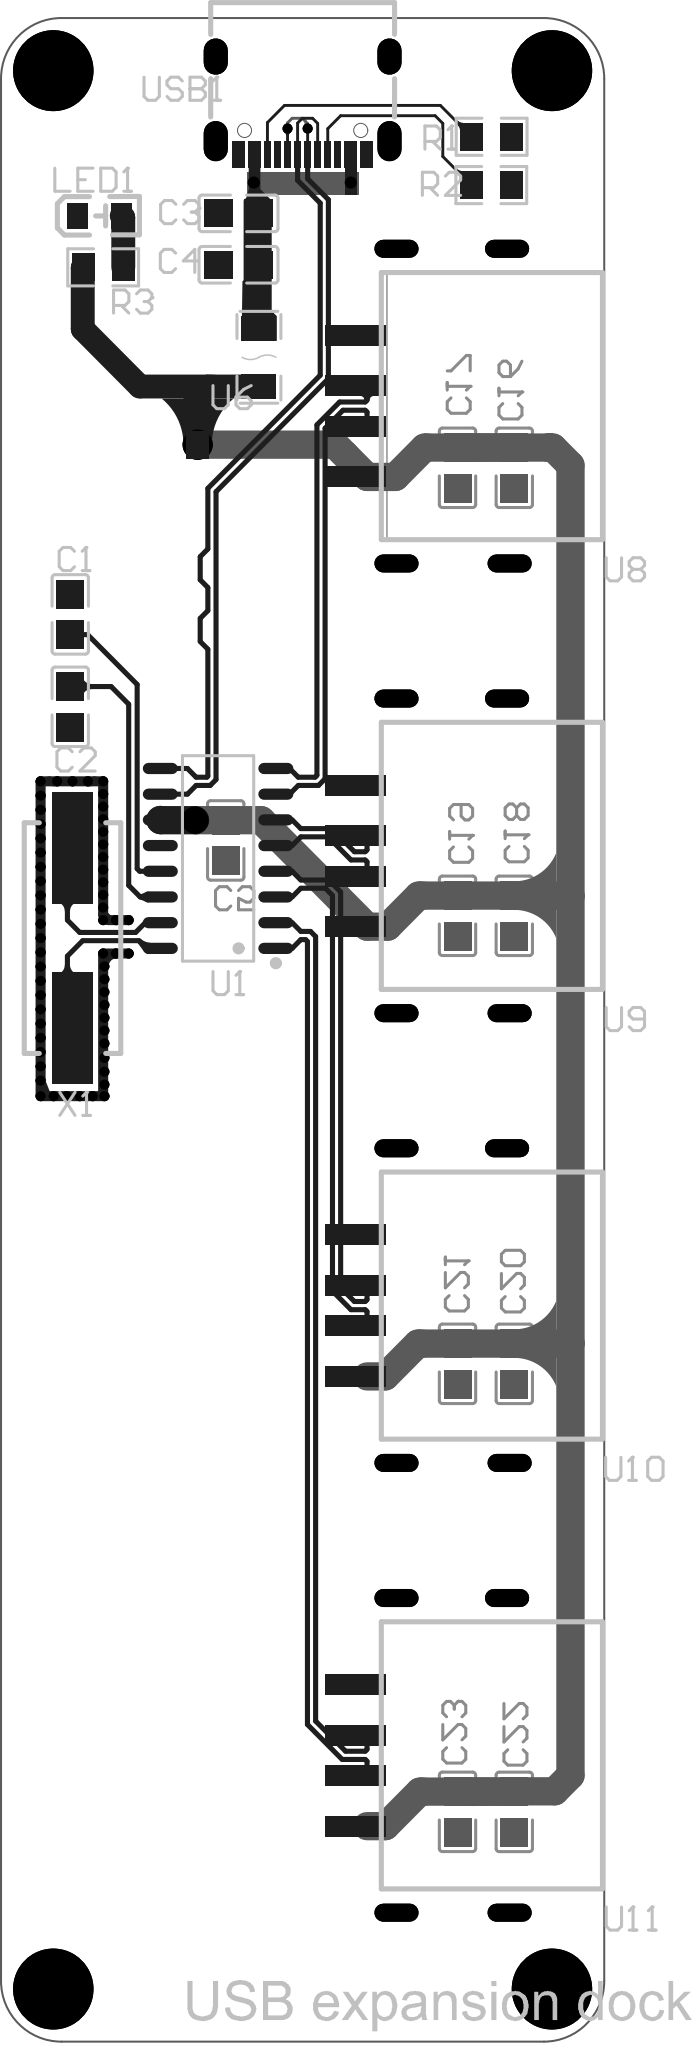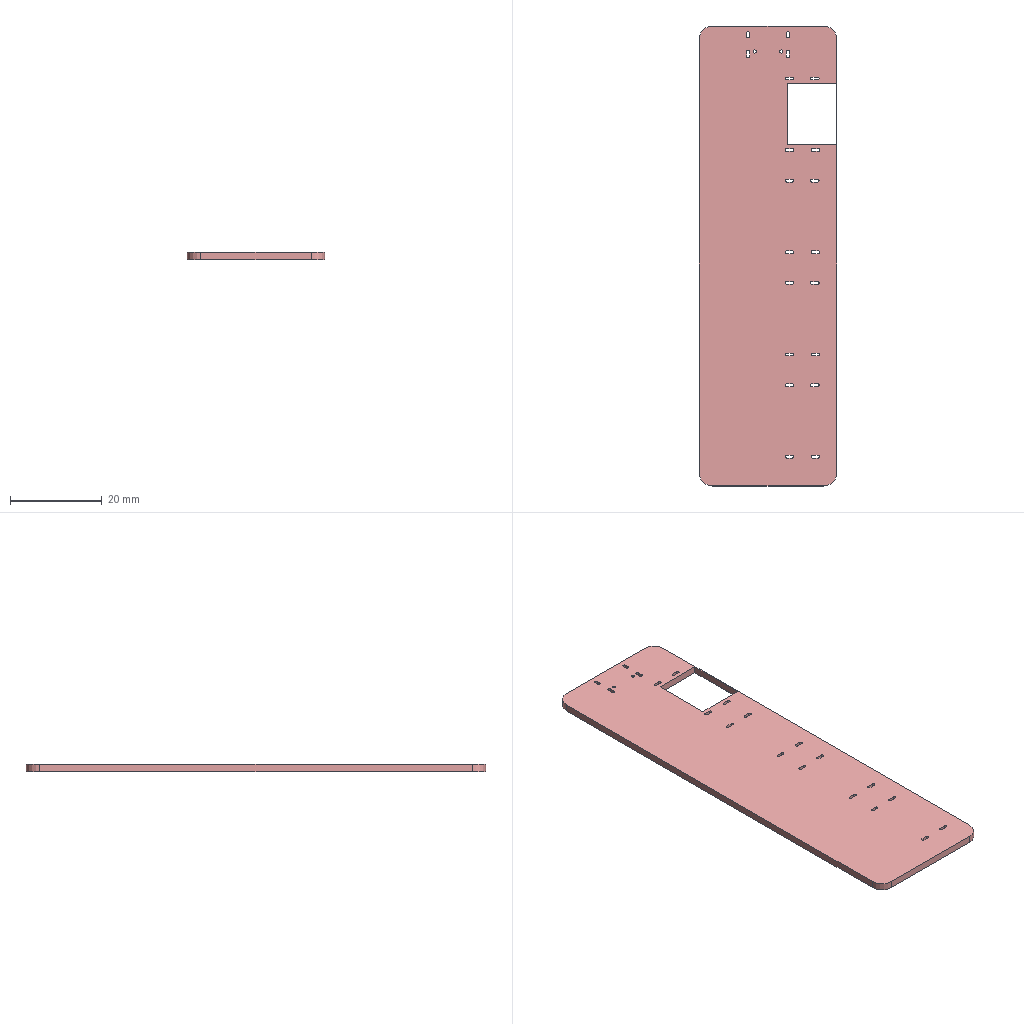Circuit board layout | Altium Designer | box 30 x 100 x 1.6 mm
Layer stack:
# Altium Designer layer stack of  (unit mm; dielectric type: 0 none, 1 core, 2 prepreg, 3 surface material)
index,name,kind,layer,copper_thickness_mm,dielectric_type,dielectric_thickness_mm,dielectric_material,dielectric_constant
0,Top Paste Mask Layer,other,,,,,,
1,Top Silkscreen Layer,other,,,,,,
2,Top Solder Mask Layer,dielectric,,,3,0.01,,3.3
3,Top Layer,copper,Top Layer,0.035,,,,
4,Dielectric1,dielectric,,,3,1.51,FR4,4.5
5,Bottom Layer,copper,Bottom Layer,0.035,,,,
6,Bottom Solder Mask Layer,dielectric,,,3,0.01,,3.3
7,Bottom Silkscreen Layer,other,,,,,,
8,Bottom Paste Mask Layer,other,,,,,,
# drill layer pairs: low layer,high layer
drill_pair,Top Layer,Bottom Layer
Part placement:
Designator,Comment,Layer,Footprint,Center-X(mm),Center-Y(mm),Rotation
U1,SL2.1A,TopLayer,SOP-16_L10.0-W3.9-P1.27-LS6.0-BL,208.534,154.432,90
USB1,typec,TopLayer,USB-C-SMD_KH-TYPE-C-16P,212.739,191.643,180
C1,100nF,TopLayer,C0805,201.182,166.491,90
C2,100nF,TopLayer,C0805,201.182,161.925,270
X1,12MHz,TopLayer,CRYSTAL-SMD_L11.1-W4.8-LS12.3,201.295,150.495,270
C3,10UF,TopLayer,C0805,209.55,186.309,0
C4,0.1UF,TopLayer,C0805,209.55,183.769,0
C5,0.1UF,BottomLayer,C0805,208.915,155.321,90
C16,10UF,BottomLayer,C0805,223.266,173.736,90
C17,0.1UF,BottomLayer,C0805,220.442,173.736,90
C18,10UF,BottomLayer,C0805,223.266,151.596,90
C19,0.1UF,BottomLayer,C0805,220.442,151.596,90
C20,10UF,BottomLayer,C0805,223.266,129.455,90
C21,0.1UF,BottomLayer,C0805,220.442,129.457,90
C22,10UF,BottomLayer,C0805,223.266,107.315,90
C23,0.1UF,BottomLayer,C0805,220.442,107.317,90
R1,5.1K,TopLayer,R0805,222.138,190.095,0
R2,5.1K,TopLayer,R0805,222.123,187.706,0
U6,1.5A快恢复保险丝-1206,TopLayer,F1206,210.566,179.197,270
R3,2K,TopLayer,R0805,202.819,183.642,180
LED1,,TopLayer,LED_0805,202.642,186.187,0
U8,USB-A-018,TopLayer,usb-smd_usb-a-018,219.202,176.784,90
U9,USB-A-018,TopLayer,usb-smd_usb-a-018,219.202,154.559,90
U10,USB-A-018,TopLayer,usb-smd_usb-a-018,219.202,132.334,90
U11,USB-A-018,TopLayer,usb-smd_usb-a-018,219.202,110.109,90
Pad and via stacks:
# Altium Designer via and pad stacks of  (unit mm). Each distinct definition once, with the count of objects using it.
# via: kind,start_layer,end_layer,hole_mm,diameter_mm,mode(0 simple;1 top-mid-bottom;2 full stack),diameter_per_layer,count,example_net
# pad: kind,layer,hole_mm,hole_type(0 round;1 square;2 slot),plating,top_size,top_shape(1 round;2 rect;3 octagon;9 rounded rect),mid_size,bottom_size,mode,footprint,size_per_layer,count,example
pad,Top Layer,0,0,plated,1.133x1.377,2,1.133x1.377,1.133x1.377,0,,,1,17
pad,Top Layer,0,0,plated,0.56x1.745,1,0.56x1.745,0.56x1.745,0,SOP-16_L10.0-W3.9-P1.27-LS6.0-BL,,16,U1.1
pad,Top Layer,0,0,plated,0.3x1.3,2,0.3x1.3,0.3x1.3,0,USB-C-SMD_KH-TYPE-C-16P,,16,USB1.A1
pad,Top Layer,0,0,plated,1.41x1.35,2,1.41x1.35,1.41x1.35,0,C0805,,8,C1.2
pad,Top Layer,0,0,plated,5.5x2,2,5.5x2,5.5x2,0,CRYSTAL-SMD_L11.1-W4.8-LS12.3,,2,X1.2
pad,Top Layer,0,0,plated,1.133x1.377,2,1.133x1.377,1.133x1.377,0,R0805,,6,R1.2
pad,Top Layer,0,0,plated,1.19x1.728,2,1.19x1.728,1.19x1.728,0,F1206,,2,U6.1
pad,Top Layer,0,0,plated,1x1.25,2,1x1.25,1x1.25,0,LED_0805,,2,LED1.2
pad,Top Layer,0,0,plated,1x3,2,1x3,1x3,0,usb-smd_usb-a-018,,16,U8.4
pad,Multi-Layer,0.7,2,plated,1.2x1.8,1,1.2x1.8,1.2x1.8,0,USB-C-SMD_KH-TYPE-C-16P,,2,USB1.3
pad,Multi-Layer,0.7,2,plated,1.2x2,1,1.2x2,1.2x2,0,USB-C-SMD_KH-TYPE-C-16P,,2,USB1.2
pad,Multi-Layer,0.6,2,plated,0.9x2.2,1,0.9x2.2,0.9x2.2,0,usb-smd_usb-a-018,,16,U8.8
pad,Bottom Layer,0,0,plated,1.41x1.35,2,1.41x1.35,1.41x1.35,0,C0805,,18,C5.2
via,Top Layer,Bottom Layer,3,4,0,,4,
via,Top Layer,Bottom Layer,1.1,1.35,0,,1,+5V
via,Top Layer,Bottom Layer,0.5004,0.6,0,,2,VCC+5V
via,Top Layer,Bottom Layer,0.3988,0.5,0,,60,DP
via,Top Layer,Bottom Layer,1.3,1.5,0,,1,+5V
Copper pours:
name,layer,net,type(0 solid;1 hatched;2 none)
Top Layer-GND,Top Layer,GND,0
Bottom Layer-GND,Bottom Layer,GND,0
Design rules, without the lines most boards share:
# Altium Designer design rules of  (exported by Altium Designer, unit mm)
# columns: name | kind | enabled | priority | scope1 | scope2 | descriptor | typed fields (field=value)
copperThickness2oz | 0 | disabled | 1 | All | All | Clearance Constraint (Gap=6mil) (Disabled)(All),(All) | gap=0.1524
Plane_innerPlane | 0 | disabled | 2 | All | All | Clearance Constraint (Gap=6mil) (Disabled)(All),(All) | gap=0.1524
Copper_copperRegion | 0 | disabled | 3 | All | All | Clearance Constraint (Gap=6mil) (Disabled)(All),(All) | gap=0.1524
copperThickness1oz | 0 | enabled | 4 | All | All | Clearance Constraint (Gap=6mil) (All),(All) | gap=0.1524
otherClearance | 52 | enabled | 1 | All | All | Hole To Hole Clearance (Gap=11.8mil) (All),(All) | gap=0.2997
viaSize | 11 | enabled | 1 | All | All | Routing Via (MinHoleWidth=11.8mil) (MaxHoleWidth=248mil) (PreferredHoleWidth=12mil) (MinWidth=19.7mil) (MaxWidth=393.7mil) (PreferedWidth=24mil) (All) | via_min_hole=0.2997 via_max_hole=6.299 via_preferred_diameter=0.6096 via_preferred_hole=0.3048